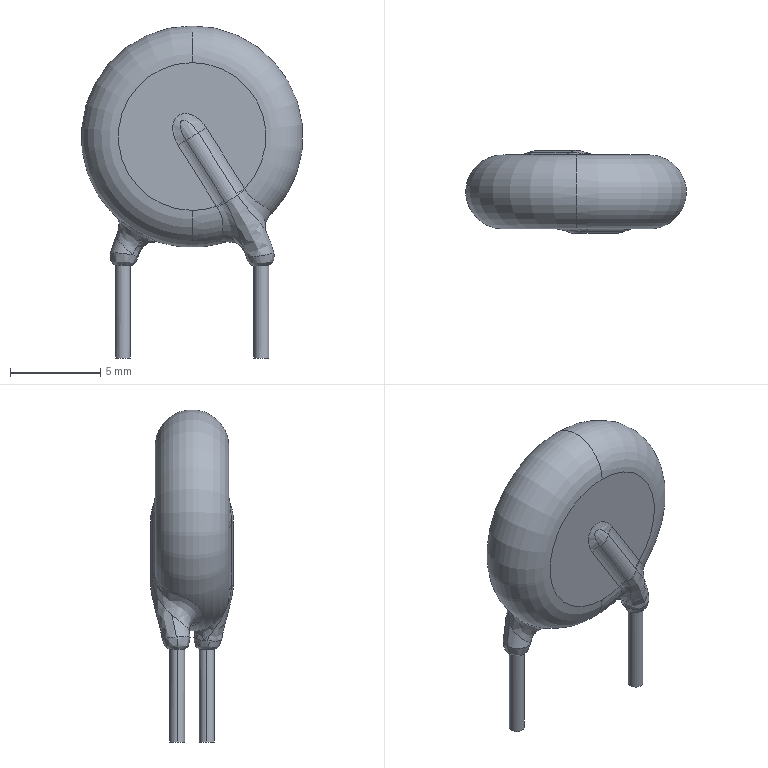Part | NX | features BREP 14 | 14 solids | 273 faces | box 12.268 x 4.6 x 18.402 mm | volume 440.129 mm3 | plane 139 | spline 122 | cylinder 10 | torus 2 | commonest cylinder face diameters 0.818 x4 2.045 x4 1.533 x2